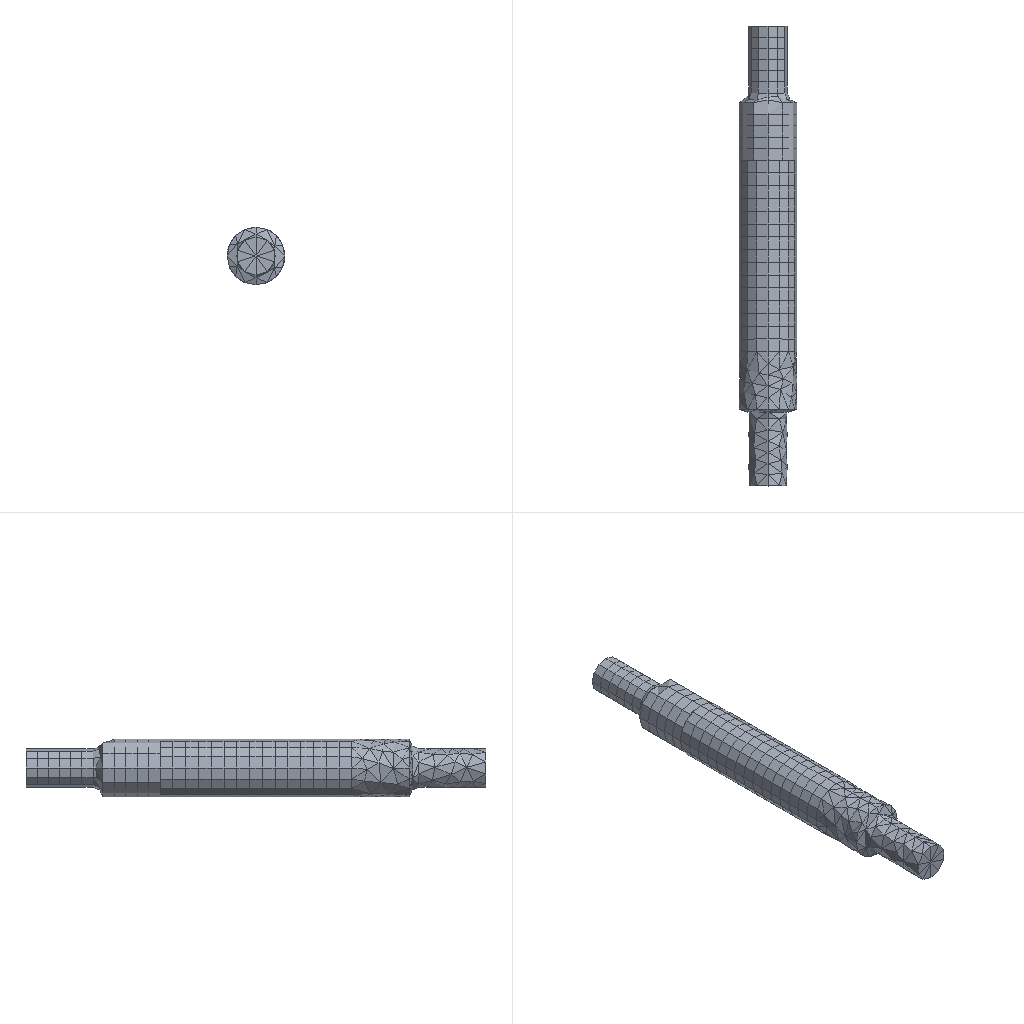Simulation study | ansys workbench
Set-up summary:
category,name,step,type,value,unit,region
solver,ansys_workbench
units,mm-N-s-tonne (MPa),,stated,"/units,MPA"
analysis,LS1,,static
load_step,LS1,LS1,static,nsubst=1; time=1
mesh,nodes,,,4710
mesh,elements,,,1435
element_type,SOLID186,,,768
element_type,SOLID187,,,439
element_type,TARGE170,,,103
element_type,CONTA174,,,103
element_type,SURF156,,,22
material,Structural Steel,,E,210000,tonne s^-2 mm^-1
material,Structural Steel,,nu,0.27
material,Structural Steel,,density,7.85e-09,tonne mm^-3
material,Structural Steel,,conductivity,60.5,tonne mm s^-3 C^-1
material,Structural Steel,,specific_heat,4.34e+08,mm^2 s^-2 C^-1
material,Structural Steel,,cte,1.2e-05,C^-1
material,Structural Steel,,permeability,10000
material,Structural Steel,,resistivity,0.00017,ohm mm
load,Define Force Using Surface Effect Elements,LS1,surface-effect pres face 1,-477.477,,SURF156 #8
load,Define Force Using Surface Effect Elements,LS1,surface-effect pres face 1,-477.49,,SURF156 #9
bc,Fixed Supports,model,fixed,[dofs=ALL],,_FIXEDSU
bc,Constant Zero Displacement X,model,fixed,[dofs=UX],,_DISPZEROUX
bc,Constant Zero Displacement Z,model,fixed,[dofs=UZ],,_DISPZEROUZ
contact,Contact Region,,bonded (always),element=CONTA174
contact,Contact Region 2,,bonded (always),element=CONTA174
named_set,_FIXEDSU,,node,32
named_set,_DISPZEROUX,,node,34
named_set,_DISPZEROUZ,,node,34
Ansys APDL input file, long lists of numbers shortened:
/batch
/config,noeldb,1     ! force off writing results to database
*get,_wallstrt,active,,time,wall
! ANSYS input file written by Workbench version 2021 R1
! File used for geometry attach:
/title,11111--____ (B5)
! ****** Begin Custom Load Command Snippet ******
/COM, ACT Extensions:
/COM,     LSDYNA, 2021.1
/COM,
! ****** End   Custom Load Command Snippet ******
*DIM,_wb_ProjectScratch_dir,string,248
_wb_ProjectScratch_dir(1) = ''
*DIM,_wb_SolverFiles_dir,string,248
_wb_SolverFiles_dir(1) = ''
*DIM,_wb_userfiles_dir,string,248
_wb_userfiles_dir(1) = ''
/com,--- Data in consistent NMM units. See Solving Units in the help system for more information.
/units,MPA
/nopr
/wb,file,start              !  signify a WB generated input file
/prep7
! Turn off shape checking because checks already performed inside WB mesher.
! See help system for more information.
SHPP,OFF,,NOWARN
/nolist
etcon,set             ! allow ANSYS to choose best KEYOP's for 180x elements, resets any applicable keyopt to MAPDL defaults
/com,*********** Nodes for the whole assembly ***********
nblock,3,,5181
(1i9,3e20.9e3)
        1    -9.103563658E+00     1.170833333E+03    -6.744736556E+00
! (4709 more lines like these left out)
-1
/wb,elem,start            !  set before creation of elements
/com,*********** Elements for Body 1 "__3-FreeParts|__-__3" ***********
et,1,186
keyo,1,2,1          ! set full integration on SOLID186
eblock,19,solid,,495
(19i9)
        1        1        1        1        0        0        0        0       20        0      713     2272     2286     2580     2552     2646     2645     2624     2626
! (989 more lines like these left out)
-1
/com,*********** Elements for Body 2 "__3-FreeParts|__2" ***********
et,2,186
keyo,2,2,1          ! set full integration on SOLID186
eblock,19,solid,,273
(19i9)
        2        2        2        2        0        0        0        0       20        0        1        5        7        8       14      191      189      188      182
! (545 more lines like these left out)
-1
/com,*********** Elements for Body 3 "__3-FreeParts|__1" ***********
et,3,187
eblock,19,solid,,439
(19i9)
        3        3        3        3        0        0        0        0       10        0      274     1406     1544     1520     1528     1660     2201     1658     1659
! (877 more lines like these left out)
-1
/wb,elem,end               !  done creating elements
/com,*********** Send User Defined Coordinate System(s) ***********
csys,0
toffst,273.15,  ! Temperature offset from absolute zero
/com,*********** Set Reference Temperature ***********
tref,22.
/wb,mat,start              !  starting to send materials
/com,*********** Send Materials ***********
Temperature = 'TEMP' ! Temperature
MP,DENS,1,7.85e-09,	! tonne mm^-3
MP,ALPX,1,1.2e-05,	! C^-1
MP,C,1,434000000,	! mm^2 s^-2 C^-1
MP,KXX,1,60.5,	! tonne mm s^-3 C^-1
MP,RSVX,1,0.00017,	! ohm mm
MP,EX,1,210000,	! tonne s^-2 mm^-1
MP,NUXY,1,0.27,
MP,MURX,1,10000,
Temperature = 'TEMP' ! Temperature
MP,DENS,2,7.85e-09,	! tonne mm^-3
MP,ALPX,2,1.2e-05,	! C^-1
MP,C,2,434000000,	! mm^2 s^-2 C^-1
MP,KXX,2,60.5,	! tonne mm s^-3 C^-1
MP,RSVX,2,0.00017,	! ohm mm
MP,EX,2,210000,	! tonne s^-2 mm^-1
MP,NUXY,2,0.27,
MP,MURX,2,10000,
Temperature = 'TEMP' ! Temperature
MP,DENS,3,7.85e-09,	! tonne mm^-3
MP,ALPX,3,1.2e-05,	! C^-1
MP,C,3,434000000,	! mm^2 s^-2 C^-1
MP,KXX,3,60.5,	! tonne mm s^-3 C^-1
MP,RSVX,3,0.00017,	! ohm mm
MP,EX,3,210000,	! tonne s^-2 mm^-1
MP,NUXY,3,0.27,
MP,MURX,3,10000,
/wb,mat,end                !  done sending materials
!************************* Model Summary ********************
!__3-FreeParts|__-__3,	结构钢,	matid,	1
!__3-FreeParts|__2,	结构钢,	matid,	2
!__3-FreeParts|__1,	结构钢,	matid,	3
!************************* End Model Summary ********************
! get the diagonal of the bounding box. Needed later for other things
*get,_xmin,node,,mnloc,x
*get,_ymin,node,,mnloc,y
*get,_zmin,node,,mnloc,z
*get,_xmax,node,,mxloc,x
*get,_ymax,node,,mxloc,y
*get,_zmax,node,,mxloc,z
_ASMDIAG=(_xmax-_xmin)*(_xmax-_xmin)+(_ymax-_ymin)*(_ymax-_ymin)+(_zmax-_zmin)*(_zmax-_zmin)
_ASMDIAG=SQRT(_ASMDIAG)
/wb,contact,start          !  starting to send contact
/com,*********** Create Contact "接触区域" ***********
/com,            Real Constant Set For Above Contact Is 5 & 4
*set,tid,5
*set,cid,4
r,tid
r,cid
et,tid,170
et,cid,174
eblock,10,,,33
(15i9)
     1976        5        5        5        0     2651     2650     2670     2670     4168     4170     2670     4173
! (32 more lines like these left out)
-1
eblock,10,,,33
(15i9)
     2009        4        4        4        0     2651     2650     2670     2670     4168     4170     2670     4173
! (32 more lines like these left out)
-1
eblock,10,,,21
(15i9)
     2042        4        5        4        0      209      200      210      210     1042     1043      210     1062
! (20 more lines like these left out)
-1
eblock,10,,,21
(15i9)
     2063        5        4        5        0      209      200      210      210     1042     1043      210     1062
! (20 more lines like these left out)
-1
keyo,cid,8,2               ! auto create asymmetric contact (from Program Controlled setting)
keyo,cid,10,0              ! adjust contact stiffness each NR iteration (from Program Controlled setting)
keyo,cid,12,5              ! bonded always
keyo,cid,18,1              ! small sliding turned on by application
keyo,cid,2,0               ! augmented Lagrange (from Program Controlled setting)
keyo,cid,4,0               ! on Gauss point (from Program Controlled setting)
keyo,cid,9,1               ! ignore initial gaps/penetration
keyo,cid,7,0               ! No Prediction
rmod,tid,3,10.      ! FKN
rmod,tid,5,0.       ! ICONT
rmod,tid,6,0.       ! PINB
rmod,tid,10,0.      ! CNOF
rmod,tid,12,0.      ! FKT
rmod,tid,36,94      ! WB DSID
rmod,cid,3,10.      ! FKN
rmod,cid,5,0.       ! ICONT
rmod,cid,6,0.       ! PINB
rmod,cid,10,0.      ! CNOF
rmod,cid,12,0.      ! FKT
rmod,cid,36,94      ! WB DSID
/com,*********** Create Contact "接触区域 2" ***********
/com,            Real Constant Set For Above Contact Is 7 & 6
*set,tid,7
*set,cid,6
r,tid
r,cid
et,tid,170
et,cid,174
eblock,10,,,33
(15i9)
     2084        7        7        7        0     2642     2623     2643     2643     4107     4108     2643     4155
! (32 more lines like these left out)
-1
eblock,10,,,33
(15i9)
     2117        6        6        6        0     2642     2623     2643     2643     4107     4108     2643     4155
! (32 more lines like these left out)
-1
eblock,10,,,16
(15i9)
     2150        6        7        6        0     1411     1412     1520     1520     1681     1689     1520     1684
! (15 more lines like these left out)
-1
eblock,10,,,16
(15i9)
     2166        7        6        7        0     1411     1412     1520     1520     1681     1689     1520     1684
! (15 more lines like these left out)
-1
keyo,cid,8,2               ! auto create asymmetric contact (from Program Controlled setting)
keyo,cid,10,0              ! adjust contact stiffness each NR iteration (from Program Controlled setting)
keyo,cid,12,5              ! bonded always
keyo,cid,18,1              ! small sliding turned on by application
keyo,cid,2,0               ! augmented Lagrange (from Program Controlled setting)
keyo,cid,4,0               ! on Gauss point (from Program Controlled setting)
keyo,cid,9,1               ! ignore initial gaps/penetration
keyo,cid,7,0               ! No Prediction
rmod,tid,3,10.      ! FKN
rmod,tid,5,0.       ! ICONT
rmod,tid,6,0.       ! PINB
rmod,tid,10,0.      ! CNOF
rmod,tid,12,0.      ! FKT
rmod,tid,36,97      ! WB DSID
rmod,cid,3,10.      ! FKN
rmod,cid,5,0.       ! ICONT
rmod,cid,6,0.       ! PINB
rmod,cid,10,0.      ! CNOF
rmod,cid,12,0.      ! FKT
rmod,cid,36,97      ! WB DSID
nsel,all
esel,all
/wb,contact,end            !  done creating contacts
/golist
/wb,load,start             !  starting to send loads
/com,*********** Fixed Supports ***********
CMBLOCK,_FIXEDSU,NODE,       32
(8i10)
      2672      2673      2674      2675      2676      2677      2678      2679
      2680      2681      2682      2683      2684      2685      2686      2687
      4215      4216      4218      4220      4222      4224      4226      4228
      4230      4232      4234      4236      4238      4240      4242      4244
cmsel,s,_FIXEDSU
d,all,all
nsel,all
/com,******* Constant Zero Displacement X *******
CMBLOCK,_DISPZEROUX,NODE,       34
(8i10)
      1405      1406      1407      1408      1409      1410      1411      1412
      1413      1649      1655      1661      1666      1671      1676      1681
      1686      2787      2794      2921      2922      2923      2924      2925
      2926      2927      4460      4468      4705      4706      4707      4708
      4709      4710
cmsel,s,_DISPZEROUX
d,all,ux,0
nsel,all
/com,******* Constant Zero Displacement Z *******
CMBLOCK,_DISPZEROUZ,NODE,       34
(8i10)
      1405      1406      1407      1408      1409      1410      1411      1412
      1413      1649      1655      1661      1666      1671      1676      1681
      1686      2787      2794      2921      2922      2923      2924      2925
      2926      2927      4460      4468      4705      4706      4707      4708
      4709      4710
cmsel,s,_DISPZEROUZ
d,all,uz,0
nsel,all
/com,*********** Define Force Using Surface Effect Elements ***********
local,12,0,0.,0.,0.,0.,0.,0.
csys,0
et,8,156
keyop,8,5,1         !  No orientation node
eblock,10,,,12
(15i9)
     2182        8        8        8       12      270      269     1200
! (11 more lines like these left out)
-1
esel,s,type,,8
keyop,8,2,1                ! Apply load in local coordinate system
keyop,8,7,1                ! Use original area so load is constant in large deformation
esel,all
/com,*********** Define Force Using Surface Effect Elements ***********
local,13,0,0.,0.,0.,0.,0.,0.
csys,0
et,9,156
keyop,9,5,1         !  No orientation node
eblock,10,,,10
(15i9)
     2194        9        9        9       13     1441     1440     1846
! (9 more lines like these left out)
-1
esel,s,type,,9
keyop,9,2,1                ! Apply load in local coordinate system
keyop,9,7,1                ! Use original area so load is constant in large deformation
esel,all
/gst,on,on
fini
*get,_numnode,node,0,count
*get,_numelem,elem,0,count
*get, _MAXELEMNUM, elem, 0, NUM, MAX
*get, _MAXNODENUM, node, 0, NUM, MAX
*get, _MAXELEMTYPE, etyp, 0, NUM, MAX
*get, _MAXREALCONST, real, 0, NUM, MAX
/go
/wb,load,end               !  done creating loads
/com,--- Number of total nodes = %_numnode%
/com,--- Number of contact elements = 228
/com,--- Number of spring elements = 0
/com,--- Number of bearing elements = 0
/com,--- Number of solid elements = 1207
/com,--- Number of condensed parts = 0
/com,--- Number of total elements = %_numelem%
*get,_wallbsol,active,,time,wall
/com,****************************************************************************
/com,*************************    SOLUTION       ********************************
/com,****************************************************************************
/solu
antype,0                   ! static analysis
_thickRatio=  1     ! Ratio of thick parts in the model
eqsl,pcg,1e-8,,,,,,1
cntr,print,1               ! print out contact info and also make no initial contact an error
dmpoption,emat,no             ! Don't combine emat file for DANSYS
dmpoption,esav,no             ! Don't combine esav file for DANSYS
nldiag,cont,iter           ! print out contact info each equilibrium iteration
rescontrol,,none                 ! Do not keep any restart files
/com,****************************************************
/com,******************* SOLVE FOR LS 1 OF 1 ****************
esel,s,type,,8
nsle
sfe,all,1,pres,1,-477.477
sfe,all,2,pres,1,0.
sfe,all,3,pres,1,0.
esel,s,type,,9
nsle
sfe,all,1,pres,1,-477.49
sfe,all,2,pres,1,0.
sfe,all,3,pres,1,0.
nsel,all
esel,all
/nopr
/gopr
/nolist
nsub,1,1,1
time,1.
outres,erase
outres,all,none
outres,nsol,all,
outres,rsol,all
outres,eangl,all
outres,etmp,all
outres,veng,all
outres,strs,all,
outres,epel,all,
outres,eppl,all,
outres,cont,all,
! *********** WB SOLVE COMMAND ***********
! check interactive state
*get,ANSINTER_,active,,int
*if,ANSINTER_,ne,0,then
/eof
*endif
solve
/com *************** Write FE CONNECTORS *********
CEWRITE,file,ce,,INTE
/com,****************************************************
/com,*************** FINISHED SOLVE FOR LS 1 *************
*get,_wallasol,active,,time,wall
/nopr
*get,_numnode,node,0,count
*get,_numelem,elem,0,count
*get, _MAXELEMNUM, elem, 0, NUM, MAX
*get, _MAXNODENUM, node, 0, NUM, MAX,,,INTERNAL
*get, _MAXELEMTYPE, etyp, 0, NUM, MAX
*get, _MAXREALCONST, real, 0, NUM, MAX
/gopr
*get,_PCGITER,active,,solu,cgiter
/post1
xmlo,ENCODING,ISO-8859-1
xmlo,parm
/xml,parm,xml
fini
/gopr
*get,_walldone,active,,time,wall
_preptime=(_wallbsol-_wallstrt)*3600
_solvtime=(_wallasol-_wallbsol)*3600
_posttime=(_walldone-_wallasol)*3600
_totaltim=(_walldone-_wallstrt)*3600
*get,_dlbratio,active,0,solu,dlbr
*get,_combtime,active,0,solu,comb
/com,--- Total number of nodes = %_numnode%
/com,--- Total number of elements = %_numelem%
/com,--- Element load balance ratio = %_dlbratio%
/com,--- Time to combine distributed files = %_combtime%
/wb,file,end               ! done with WB generated input
Results summary:
result,analyses[0].index,,,1
result,analyses[0].system,,,SYS
result,analyses[0].deck,,,deck.dat
result,analyses[0].solve_status,,,completed
result,analyses[0].analysis_type,,,static
result,analyses[0].physics,,,mechanical
result,analyses[0].unit_system,,,"NMM: mm, ton, N, s, mV, mA, degC"
result,analyses[0].n_sets,,,1
result,analyses[0].load_steps[0].set,set=1,,1
result,analyses[0].load_steps[0].time_or_freq,set=1,,1
result,analyses[0].load_steps[0].max_displacement_magnitude,set=1,,1.331
result,analyses[0].load_steps[0].max_von_mises_nodal,set=1,,370.225
result,analyses[0].load_steps[0].reaction_force_sum_xyz[1],set=1,,299977
result,analyses[0].load_steps[0].reaction_force_sum_xyz[2],set=1,,0.001893
result,analyses[0].load_steps[0].reaction_force_sum_xyz[3],set=1,,-0.00929